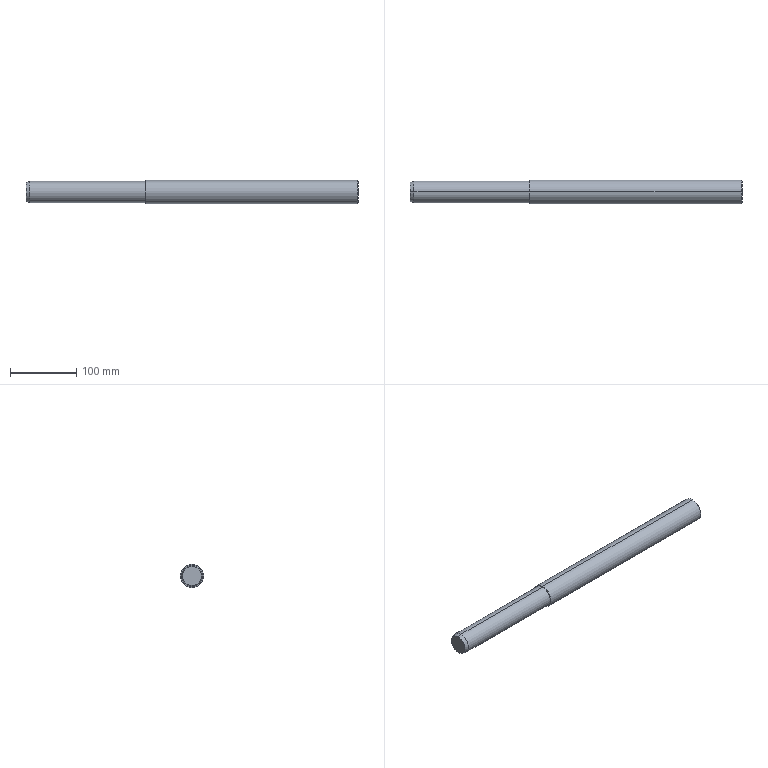Part | SolidWorks | features MBimport 1 | 1 solid | 20 faces | box 500 x 35 x 35 mm | volume 451710 mm3 | cone 8 | cylinder 8 | plane 4 | commonest cylinder face diameters 5 x2 6 x2 32 x2 35 x2
STEP:
#1=CARTESIAN_POINT('',(-0.025,10.786,1.92));
#2=VERTEX_POINT('',#1);
#3=CARTESIAN_POINT('',(0.,10.786,1.945));
#4=VERTEX_POINT('',#3);
#5=CARTESIAN_POINT('',(0.,10.786,1.945));
#6=DIRECTION('',(0.7071,0.,0.7071));
#7=VECTOR('',#6,1000.);
#8=LINE('',#5,#7);
#9=EDGE_CURVE('',#2,#4,#8,.T.);
#10=ORIENTED_EDGE('',*,*,#9,.F.);
#11=CARTESIAN_POINT('',(-0.025,10.786,-4.08));
#12=VERTEX_POINT('',#11);
#13=CARTESIAN_POINT('',(-0.025,10.786,-1.08));
#14=DIRECTION('',(1.,0.,0.));
#15=DIRECTION('',(0.,0.,-1.));
#16=AXIS2_PLACEMENT_3D('',#13,#14,#15);
#17=CIRCLE('',#16,3.);
#18=EDGE_CURVE('',#12,#2,#17,.T.);
#19=ORIENTED_EDGE('',*,*,#18,.F.);
#20=CARTESIAN_POINT('',(0.,10.786,-4.105));
#21=VERTEX_POINT('',#20);
#22=CARTESIAN_POINT('',(0.,10.786,-4.105));
#23=DIRECTION('',(0.7071,0.,-0.7071));
#24=VECTOR('',#23,1000.);
#25=LINE('',#22,#24);
#26=EDGE_CURVE('',#12,#21,#25,.T.);
#27=ORIENTED_EDGE('',*,*,#26,.T.);
#28=CARTESIAN_POINT('',(0.,10.786,-1.08));
#29=DIRECTION('',(1.,0.,0.));
#30=DIRECTION('',(0.,0.,-1.));
#31=AXIS2_PLACEMENT_3D('',#28,#29,#30);
#32=CIRCLE('',#31,3.025);
#33=EDGE_CURVE('',#21,#4,#32,.T.);
#34=ORIENTED_EDGE('',*,*,#33,.T.);
#35=EDGE_LOOP('',(#10,#19,#27,#34));
#36=FACE_OUTER_BOUND('',#35,.T.);
#37=CARTESIAN_POINT('',(0.,10.786,-1.08));
#38=DIRECTION('',(1.,0.,0.));
#39=DIRECTION('',(0.,0.,-1.));
#40=AXIS2_PLACEMENT_3D('',#37,#38,#39);
#41=CONICAL_SURFACE('',#40,3.025,0.7854);
#42=ADVANCED_FACE('',(#36),#41,.F.);
#43=CARTESIAN_POINT('',(-12.,10.786,1.92));
#44=VERTEX_POINT('',#43);
#45=CARTESIAN_POINT('',(0.,10.786,1.92));
#46=DIRECTION('',(1.,0.,0.));
#47=VECTOR('',#46,1000.);
#48=LINE('',#45,#47);
#49=EDGE_CURVE('',#44,#2,#48,.T.);
#50=ORIENTED_EDGE('',*,*,#49,.F.);
#51=CARTESIAN_POINT('',(-12.,10.786,-4.08));
#52=VERTEX_POINT('',#51);
#53=CARTESIAN_POINT('',(-12.,10.786,-1.08));
#54=DIRECTION('',(1.,0.,0.));
#55=DIRECTION('',(0.,0.,-1.));
#56=AXIS2_PLACEMENT_3D('',#53,#54,#55);
#57=CIRCLE('',#56,3.);
#58=EDGE_CURVE('',#52,#44,#57,.T.);
#59=ORIENTED_EDGE('',*,*,#58,.F.);
#60=CARTESIAN_POINT('',(0.,10.786,-4.08));
#61=DIRECTION('',(1.,0.,0.));
#62=VECTOR('',#61,1000.);
#63=LINE('',#60,#62);
#64=EDGE_CURVE('',#52,#12,#63,.T.);
#65=ORIENTED_EDGE('',*,*,#64,.T.);
#66=ORIENTED_EDGE('',*,*,#18,.T.);
#67=EDGE_LOOP('',(#50,#59,#65,#66));
#68=FACE_OUTER_BOUND('',#67,.T.);
#69=CARTESIAN_POINT('',(0.,10.786,-1.08));
#70=DIRECTION('',(1.,0.,0.));
#71=DIRECTION('',(0.,0.,-1.));
#72=AXIS2_PLACEMENT_3D('',#69,#70,#71);
#73=CYLINDRICAL_SURFACE('',#72,3.);
#74=ADVANCED_FACE('',(#68),#73,.F.);
#75=CARTESIAN_POINT('',(-12.,10.786,-3.58));
#76=VERTEX_POINT('',#75);
#77=CARTESIAN_POINT('',(-12.,10.786,1.42));
#78=VERTEX_POINT('',#77);
#79=CARTESIAN_POINT('',(-12.,10.786,-1.08));
#80=DIRECTION('',(1.,0.,0.));
#81=DIRECTION('',(0.,0.,-1.));
#82=AXIS2_PLACEMENT_3D('',#79,#80,#81);
#83=CIRCLE('',#82,2.5);
#84=EDGE_CURVE('',#76,#78,#83,.T.);
#85=ORIENTED_EDGE('',*,*,#84,.F.);
#86=CARTESIAN_POINT('',(-12.,10.786,-1.08));
#87=DIRECTION('',(1.,0.,0.));
#88=DIRECTION('',(0.,0.,-1.));
#89=AXIS2_PLACEMENT_3D('',#86,#87,#88);
#90=CIRCLE('',#89,2.5);
#91=EDGE_CURVE('',#78,#76,#90,.T.);
#92=ORIENTED_EDGE('',*,*,#91,.F.);
#93=EDGE_LOOP('',(#85,#92));
#94=FACE_BOUND('',#93,.T.);
#95=ORIENTED_EDGE('',*,*,#58,.T.);
#96=CARTESIAN_POINT('',(-12.,10.786,-1.08));
#97=DIRECTION('',(1.,0.,0.));
#98=DIRECTION('',(0.,0.,-1.));
#99=AXIS2_PLACEMENT_3D('',#96,#97,#98);
#100=CIRCLE('',#99,3.);
#101=EDGE_CURVE('',#44,#52,#100,.T.);
#102=ORIENTED_EDGE('',*,*,#101,.T.);
#103=EDGE_LOOP('',(#95,#102));
#104=FACE_OUTER_BOUND('',#103,.T.);
#105=CARTESIAN_POINT('',(-12.,13.286,-1.08));
#106=DIRECTION('',(-1.,0.,0.));
#107=DIRECTION('',(0.,0.,1.));
#108=AXIS2_PLACEMENT_3D('',#105,#106,#107);
#109=PLANE('',#108);
#110=ADVANCED_FACE('',(#94,#104),#109,.F.);
#111=CARTESIAN_POINT('',(-15.,10.786,1.42));
#112=VERTEX_POINT('',#111);
#113=CARTESIAN_POINT('',(0.,10.786,1.42));
#114=DIRECTION('',(1.,0.,0.));
#115=VECTOR('',#114,1000.);
#116=LINE('',#113,#115);
#117=EDGE_CURVE('',#112,#78,#116,.T.);
#118=ORIENTED_EDGE('',*,*,#117,.F.);
#119=CARTESIAN_POINT('',(-15.,10.786,-3.58));
#120=VERTEX_POINT('',#119);
#121=CARTESIAN_POINT('',(-15.,10.786,-1.08));
#122=DIRECTION('',(1.,0.,0.));
#123=DIRECTION('',(0.,0.,-1.));
#124=AXIS2_PLACEMENT_3D('',#121,#122,#123);
#125=CIRCLE('',#124,2.5);
#126=EDGE_CURVE('',#120,#112,#125,.T.);
#127=ORIENTED_EDGE('',*,*,#126,.F.);
#128=CARTESIAN_POINT('',(0.,10.786,-3.58));
#129=DIRECTION('',(1.,0.,0.));
#130=VECTOR('',#129,1000.);
#131=LINE('',#128,#130);
#132=EDGE_CURVE('',#120,#76,#131,.T.);
#133=ORIENTED_EDGE('',*,*,#132,.T.);
#134=ORIENTED_EDGE('',*,*,#84,.T.);
#135=EDGE_LOOP('',(#118,#127,#133,#134));
#136=FACE_OUTER_BOUND('',#135,.T.);
#137=CARTESIAN_POINT('',(0.,10.786,-1.08));
#138=DIRECTION('',(1.,0.,0.));
#139=DIRECTION('',(0.,0.,-1.));
#140=AXIS2_PLACEMENT_3D('',#137,#138,#139);
#141=CYLINDRICAL_SURFACE('',#140,2.5);
#142=ADVANCED_FACE('',(#136),#141,.F.);
#143=CARTESIAN_POINT('',(-16.502,10.786,-1.08));
#144=VERTEX_POINT('',#143);
#145=CARTESIAN_POINT('',(-15.,10.786,1.42));
#146=DIRECTION('',(0.515,0.,0.8572));
#147=VECTOR('',#146,1000.);
#148=LINE('',#145,#147);
#149=EDGE_CURVE('',#144,#112,#148,.T.);
#150=ORIENTED_EDGE('',*,*,#149,.F.);
#151=CARTESIAN_POINT('',(-15.,10.786,-3.58));
#152=DIRECTION('',(0.515,0.,-0.8572));
#153=VECTOR('',#152,1000.);
#154=LINE('',#151,#153);
#155=EDGE_CURVE('',#144,#120,#154,.T.);
#156=ORIENTED_EDGE('',*,*,#155,.T.);
#157=ORIENTED_EDGE('',*,*,#126,.T.);
#158=EDGE_LOOP('',(#150,#156,#157));
#159=FACE_OUTER_BOUND('',#158,.T.);
#160=CARTESIAN_POINT('',(-15.,10.786,-1.08));
#161=DIRECTION('',(1.,0.,0.));
#162=DIRECTION('',(0.,0.,-1.));
#163=AXIS2_PLACEMENT_3D('',#160,#161,#162);
#164=CONICAL_SURFACE('',#163,2.5,1.03);
#165=ADVANCED_FACE('',(#159),#164,.F.);
#166=CARTESIAN_POINT('',(0.,10.786,-17.58));
#167=VERTEX_POINT('',#166);
#168=CARTESIAN_POINT('',(-1.,10.786,-18.58));
#169=VERTEX_POINT('',#168);
#170=CARTESIAN_POINT('',(0.,10.786,-17.58));
#171=DIRECTION('',(-0.7071,0.,-0.7071));
#172=VECTOR('',#171,1000.);
#173=LINE('',#170,#172);
#174=EDGE_CURVE('',#167,#169,#173,.T.);
#175=ORIENTED_EDGE('',*,*,#174,.F.);
#176=CARTESIAN_POINT('',(0.,10.786,15.42));
#177=VERTEX_POINT('',#176);
#178=CARTESIAN_POINT('',(0.,10.786,-1.08));
#179=DIRECTION('',(1.,0.,0.));
#180=DIRECTION('',(0.,0.,-1.));
#181=AXIS2_PLACEMENT_3D('',#178,#179,#180);
#182=CIRCLE('',#181,16.5);
#183=EDGE_CURVE('',#177,#167,#182,.T.);
#184=ORIENTED_EDGE('',*,*,#183,.F.);
#185=CARTESIAN_POINT('',(-1.,10.786,16.42));
#186=VERTEX_POINT('',#185);
#187=CARTESIAN_POINT('',(0.,10.786,15.42));
#188=DIRECTION('',(-0.7071,0.,0.7071));
#189=VECTOR('',#188,1000.);
#190=LINE('',#187,#189);
#191=EDGE_CURVE('',#177,#186,#190,.T.);
#192=ORIENTED_EDGE('',*,*,#191,.T.);
#193=CARTESIAN_POINT('',(-1.,10.786,-1.08));
#194=DIRECTION('',(-1.,0.,0.));
#195=DIRECTION('',(0.,0.,-1.));
#196=AXIS2_PLACEMENT_3D('',#193,#194,#195);
#197=CIRCLE('',#196,17.5);
#198=EDGE_CURVE('',#169,#186,#197,.T.);
#199=ORIENTED_EDGE('',*,*,#198,.F.);
#200=EDGE_LOOP('',(#175,#184,#192,#199));
#201=FACE_OUTER_BOUND('',#200,.T.);
#202=CARTESIAN_POINT('',(0.,10.786,-1.08));
#203=DIRECTION('',(-1.,0.,0.));
#204=DIRECTION('',(0.,0.,1.));
#205=AXIS2_PLACEMENT_3D('',#202,#203,#204);
#206=CONICAL_SURFACE('',#205,16.5,0.7854);
#207=ADVANCED_FACE('',(#201),#206,.T.);
#208=CARTESIAN_POINT('',(-500.,10.786,13.313));
#209=VERTEX_POINT('',#208);
#210=CARTESIAN_POINT('',(-494.,10.786,14.92));
#211=VERTEX_POINT('',#210);
#212=CARTESIAN_POINT('',(-500.,10.786,13.313));
#213=DIRECTION('',(0.9659,0.,0.2588));
#214=VECTOR('',#213,1000.);
#215=LINE('',#212,#214);
#216=EDGE_CURVE('',#209,#211,#215,.T.);
#217=ORIENTED_EDGE('',*,*,#216,.F.);
#218=CARTESIAN_POINT('',(-500.,10.786,-15.472));
#219=VERTEX_POINT('',#218);
#220=CARTESIAN_POINT('',(-500.,10.786,-1.08));
#221=DIRECTION('',(-1.,0.,0.));
#222=DIRECTION('',(0.,0.,1.));
#223=AXIS2_PLACEMENT_3D('',#220,#221,#222);
#224=CIRCLE('',#223,14.392);
#225=EDGE_CURVE('',#219,#209,#224,.T.);
#226=ORIENTED_EDGE('',*,*,#225,.F.);
#227=CARTESIAN_POINT('',(-494.,10.786,-17.08));
#228=VERTEX_POINT('',#227);
#229=CARTESIAN_POINT('',(-500.,10.786,-15.472));
#230=DIRECTION('',(0.9659,0.,-0.2588));
#231=VECTOR('',#230,1000.);
#232=LINE('',#229,#231);
#233=EDGE_CURVE('',#219,#228,#232,.T.);
#234=ORIENTED_EDGE('',*,*,#233,.T.);
#235=CARTESIAN_POINT('',(-494.,10.786,-1.08));
#236=DIRECTION('',(1.,0.,0.));
#237=DIRECTION('',(0.,0.,1.));
#238=AXIS2_PLACEMENT_3D('',#235,#236,#237);
#239=CIRCLE('',#238,16.);
#240=EDGE_CURVE('',#211,#228,#239,.T.);
#241=ORIENTED_EDGE('',*,*,#240,.F.);
#242=EDGE_LOOP('',(#217,#226,#234,#241));
#243=FACE_OUTER_BOUND('',#242,.T.);
#244=CARTESIAN_POINT('',(-500.,10.786,-1.08));
#245=DIRECTION('',(1.,0.,0.));
#246=DIRECTION('',(0.,0.,-1.));
#247=AXIS2_PLACEMENT_3D('',#244,#245,#246);
#248=CONICAL_SURFACE('',#247,14.392,0.2618);
#249=ADVANCED_FACE('',(#243),#248,.T.);
#250=ORIENTED_EDGE('',*,*,#225,.T.);
#251=CARTESIAN_POINT('',(-500.,10.786,-1.08));
#252=DIRECTION('',(-1.,0.,0.));
#253=DIRECTION('',(0.,0.,1.));
#254=AXIS2_PLACEMENT_3D('',#251,#252,#253);
#255=CIRCLE('',#254,14.392);
#256=EDGE_CURVE('',#209,#219,#255,.T.);
#257=ORIENTED_EDGE('',*,*,#256,.T.);
#258=EDGE_LOOP('',(#250,#257));
#259=FACE_OUTER_BOUND('',#258,.T.);
#260=CARTESIAN_POINT('',(-500.,10.786,-1.08));
#261=DIRECTION('',(-1.,0.,0.));
#262=DIRECTION('',(0.,0.,1.));
#263=AXIS2_PLACEMENT_3D('',#260,#261,#262);
#264=PLANE('',#263);
#265=ADVANCED_FACE('',(#259),#264,.T.);
#266=CARTESIAN_POINT('',(-320.,10.786,14.92));
#267=VERTEX_POINT('',#266);
#268=CARTESIAN_POINT('',(-500.,10.786,14.92));
#269=DIRECTION('',(1.,0.,0.));
#270=VECTOR('',#269,1000.);
#271=LINE('',#268,#270);
#272=EDGE_CURVE('',#211,#267,#271,.T.);
#273=ORIENTED_EDGE('',*,*,#272,.F.);
#274=ORIENTED_EDGE('',*,*,#240,.T.);
#275=CARTESIAN_POINT('',(-320.,10.786,-17.08));
#276=VERTEX_POINT('',#275);
#277=CARTESIAN_POINT('',(-500.,10.786,-17.08));
#278=DIRECTION('',(1.,0.,0.));
#279=VECTOR('',#278,1000.);
#280=LINE('',#277,#279);
#281=EDGE_CURVE('',#228,#276,#280,.T.);
#282=ORIENTED_EDGE('',*,*,#281,.T.);
#283=CARTESIAN_POINT('',(-320.,10.786,-1.08));
#284=DIRECTION('',(-1.,0.,0.));
#285=DIRECTION('',(0.,0.,1.));
#286=AXIS2_PLACEMENT_3D('',#283,#284,#285);
#287=CIRCLE('',#286,16.);
#288=EDGE_CURVE('',#276,#267,#287,.T.);
#289=ORIENTED_EDGE('',*,*,#288,.T.);
#290=EDGE_LOOP('',(#273,#274,#282,#289));
#291=FACE_OUTER_BOUND('',#290,.T.);
#292=CARTESIAN_POINT('',(-500.,10.786,-1.08));
#293=DIRECTION('',(1.,0.,0.));
#294=DIRECTION('',(0.,0.,-1.));
#295=AXIS2_PLACEMENT_3D('',#292,#293,#294);
#296=CYLINDRICAL_SURFACE('',#295,16.);
#297=ADVANCED_FACE('',(#291),#296,.T.);
#298=ORIENTED_EDGE('',*,*,#33,.F.);
#299=CARTESIAN_POINT('',(0.,10.786,-1.08));
#300=DIRECTION('',(1.,0.,0.));
#301=DIRECTION('',(0.,0.,-1.));
#302=AXIS2_PLACEMENT_3D('',#299,#300,#301);
#303=CIRCLE('',#302,3.025);
#304=EDGE_CURVE('',#4,#21,#303,.T.);
#305=ORIENTED_EDGE('',*,*,#304,.F.);
#306=EDGE_LOOP('',(#298,#305));
#307=FACE_BOUND('',#306,.T.);
#308=ORIENTED_EDGE('',*,*,#183,.T.);
#309=CARTESIAN_POINT('',(0.,10.786,-1.08));
#310=DIRECTION('',(1.,0.,0.));
#311=DIRECTION('',(0.,0.,-1.));
#312=AXIS2_PLACEMENT_3D('',#309,#310,#311);
#313=CIRCLE('',#312,16.5);
#314=EDGE_CURVE('',#167,#177,#313,.T.);
#315=ORIENTED_EDGE('',*,*,#314,.T.);
#316=EDGE_LOOP('',(#308,#315));
#317=FACE_OUTER_BOUND('',#316,.T.);
#318=CARTESIAN_POINT('',(0.,10.786,-1.08));
#319=DIRECTION('',(1.,0.,0.));
#320=DIRECTION('',(0.,1.,0.));
#321=AXIS2_PLACEMENT_3D('',#318,#319,#320);
#322=PLANE('',#321);
#323=ADVANCED_FACE('',(#307,#317),#322,.T.);
#324=ORIENTED_EDGE('',*,*,#288,.F.);
#325=CARTESIAN_POINT('',(-320.,10.786,-1.08));
#326=DIRECTION('',(-1.,0.,0.));
#327=DIRECTION('',(0.,0.,1.));
#328=AXIS2_PLACEMENT_3D('',#325,#326,#327);
#329=CIRCLE('',#328,16.);
#330=EDGE_CURVE('',#267,#276,#329,.T.);
#331=ORIENTED_EDGE('',*,*,#330,.F.);
#332=EDGE_LOOP('',(#324,#331));
#333=FACE_BOUND('',#332,.T.);
#334=CARTESIAN_POINT('',(-320.,10.786,-18.58));
#335=VERTEX_POINT('',#334);
#336=CARTESIAN_POINT('',(-320.,10.786,16.42));
#337=VERTEX_POINT('',#336);
#338=CARTESIAN_POINT('',(-320.,10.786,-1.08));
#339=DIRECTION('',(1.,0.,0.));
#340=DIRECTION('',(0.,0.,-1.));
#341=AXIS2_PLACEMENT_3D('',#338,#339,#340);
#342=CIRCLE('',#341,17.5);
#343=EDGE_CURVE('',#335,#337,#342,.T.);
#344=ORIENTED_EDGE('',*,*,#343,.F.);
#345=CARTESIAN_POINT('',(-320.,10.786,-1.08));
#346=DIRECTION('',(1.,0.,0.));
#347=DIRECTION('',(0.,0.,-1.));
#348=AXIS2_PLACEMENT_3D('',#345,#346,#347);
#349=CIRCLE('',#348,17.5);
#350=EDGE_CURVE('',#337,#335,#349,.T.);
#351=ORIENTED_EDGE('',*,*,#350,.F.);
#352=EDGE_LOOP('',(#344,#351));
#353=FACE_OUTER_BOUND('',#352,.T.);
#354=CARTESIAN_POINT('',(-320.,10.786,-1.08));
#355=DIRECTION('',(1.,0.,0.));
#356=DIRECTION('',(0.,1.,0.));
#357=AXIS2_PLACEMENT_3D('',#354,#355,#356);
#358=PLANE('',#357);
#359=ADVANCED_FACE('',(#333,#353),#358,.F.);
#360=CARTESIAN_POINT('',(-320.,10.786,16.42));
#361=DIRECTION('',(1.,0.,0.));
#362=VECTOR('',#361,1000.);
#363=LINE('',#360,#362);
#364=EDGE_CURVE('',#337,#186,#363,.T.);
#365=ORIENTED_EDGE('',*,*,#364,.F.);
#366=ORIENTED_EDGE('',*,*,#350,.T.);
#367=CARTESIAN_POINT('',(-320.,10.786,-18.58));
#368=DIRECTION('',(1.,0.,0.));
#369=VECTOR('',#368,1000.);
#370=LINE('',#367,#369);
#371=EDGE_CURVE('',#335,#169,#370,.T.);
#372=ORIENTED_EDGE('',*,*,#371,.T.);
#373=ORIENTED_EDGE('',*,*,#198,.T.);
#374=EDGE_LOOP('',(#365,#366,#372,#373));
#375=FACE_OUTER_BOUND('',#374,.T.);
#376=CARTESIAN_POINT('',(-320.,10.786,-1.08));
#377=DIRECTION('',(1.,0.,0.));
#378=DIRECTION('',(0.,0.,-1.));
#379=AXIS2_PLACEMENT_3D('',#376,#377,#378);
#380=CYLINDRICAL_SURFACE('',#379,17.5);
#381=ADVANCED_FACE('',(#375),#380,.T.);
#382=ORIENTED_EDGE('',*,*,#343,.T.);
#383=ORIENTED_EDGE('',*,*,#364,.T.);
#384=CARTESIAN_POINT('',(-1.,10.786,-1.08));
#385=DIRECTION('',(-1.,0.,0.));
#386=DIRECTION('',(0.,0.,-1.));
#387=AXIS2_PLACEMENT_3D('',#384,#385,#386);
#388=CIRCLE('',#387,17.5);
#389=EDGE_CURVE('',#186,#169,#388,.T.);
#390=ORIENTED_EDGE('',*,*,#389,.T.);
#391=ORIENTED_EDGE('',*,*,#371,.F.);
#392=EDGE_LOOP('',(#382,#383,#390,#391));
#393=FACE_OUTER_BOUND('',#392,.T.);
#394=CARTESIAN_POINT('',(-320.,10.786,-1.08));
#395=DIRECTION('',(1.,0.,0.));
#396=DIRECTION('',(0.,0.,-1.));
#397=AXIS2_PLACEMENT_3D('',#394,#395,#396);
#398=CYLINDRICAL_SURFACE('',#397,17.5);
#399=ADVANCED_FACE('',(#393),#398,.T.);
#400=CARTESIAN_POINT('',(-494.,10.786,-1.08));
#401=DIRECTION('',(1.,0.,0.));
#402=DIRECTION('',(0.,0.,1.));
#403=AXIS2_PLACEMENT_3D('',#400,#401,#402);
#404=CIRCLE('',#403,16.);
#405=EDGE_CURVE('',#228,#211,#404,.T.);
#406=ORIENTED_EDGE('',*,*,#405,.T.);
#407=ORIENTED_EDGE('',*,*,#272,.T.);
#408=ORIENTED_EDGE('',*,*,#330,.T.);
#409=ORIENTED_EDGE('',*,*,#281,.F.);
#410=EDGE_LOOP('',(#406,#407,#408,#409));
#411=FACE_OUTER_BOUND('',#410,.T.);
#412=CARTESIAN_POINT('',(-500.,10.786,-1.08));
#413=DIRECTION('',(1.,0.,0.));
#414=DIRECTION('',(0.,0.,-1.));
#415=AXIS2_PLACEMENT_3D('',#412,#413,#414);
#416=CYLINDRICAL_SURFACE('',#415,16.);
#417=ADVANCED_FACE('',(#411),#416,.T.);
#418=ORIENTED_EDGE('',*,*,#256,.F.);
#419=ORIENTED_EDGE('',*,*,#216,.T.);
#420=ORIENTED_EDGE('',*,*,#405,.F.);
#421=ORIENTED_EDGE('',*,*,#233,.F.);
#422=EDGE_LOOP('',(#418,#419,#420,#421));
#423=FACE_OUTER_BOUND('',#422,.T.);
#424=CARTESIAN_POINT('',(-500.,10.786,-1.08));
#425=DIRECTION('',(1.,0.,0.));
#426=DIRECTION('',(0.,0.,-1.));
#427=AXIS2_PLACEMENT_3D('',#424,#425,#426);
#428=CONICAL_SURFACE('',#427,14.392,0.2618);
#429=ADVANCED_FACE('',(#423),#428,.T.);
#430=ORIENTED_EDGE('',*,*,#314,.F.);
#431=ORIENTED_EDGE('',*,*,#174,.T.);
#432=ORIENTED_EDGE('',*,*,#389,.F.);
#433=ORIENTED_EDGE('',*,*,#191,.F.);
#434=EDGE_LOOP('',(#430,#431,#432,#433));
#435=FACE_OUTER_BOUND('',#434,.T.);
#436=CARTESIAN_POINT('',(0.,10.786,-1.08));
#437=DIRECTION('',(-1.,0.,0.));
#438=DIRECTION('',(0.,0.,1.));
#439=AXIS2_PLACEMENT_3D('',#436,#437,#438);
#440=CONICAL_SURFACE('',#439,16.5,0.7854);
#441=ADVANCED_FACE('',(#435),#440,.T.);
#442=ORIENTED_EDGE('',*,*,#155,.F.);
#443=ORIENTED_EDGE('',*,*,#149,.T.);
#444=CARTESIAN_POINT('',(-15.,10.786,-1.08));
#445=DIRECTION('',(1.,0.,0.));
#446=DIRECTION('',(0.,0.,-1.));
#447=AXIS2_PLACEMENT_3D('',#444,#445,#446);
#448=CIRCLE('',#447,2.5);
#449=EDGE_CURVE('',#112,#120,#448,.T.);
#450=ORIENTED_EDGE('',*,*,#449,.T.);
#451=EDGE_LOOP('',(#442,#443,#450));
#452=FACE_OUTER_BOUND('',#451,.T.);
#453=CARTESIAN_POINT('',(-15.,10.786,-1.08));
#454=DIRECTION('',(1.,0.,0.));
#455=DIRECTION('',(0.,0.,-1.));
#456=AXIS2_PLACEMENT_3D('',#453,#454,#455);
#457=CONICAL_SURFACE('',#456,2.5,1.03);
#458=ADVANCED_FACE('',(#452),#457,.F.);
#459=ORIENTED_EDGE('',*,*,#449,.F.);
#460=ORIENTED_EDGE('',*,*,#117,.T.);
#461=ORIENTED_EDGE('',*,*,#91,.T.);
#462=ORIENTED_EDGE('',*,*,#132,.F.);
#463=EDGE_LOOP('',(#459,#460,#461,#462));
#464=FACE_OUTER_BOUND('',#463,.T.);
#465=CARTESIAN_POINT('',(0.,10.786,-1.08));
#466=DIRECTION('',(1.,0.,0.));
#467=DIRECTION('',(0.,0.,-1.));
#468=AXIS2_PLACEMENT_3D('',#465,#466,#467);
#469=CYLINDRICAL_SURFACE('',#468,2.5);
#470=ADVANCED_FACE('',(#464),#469,.F.);
#471=ORIENTED_EDGE('',*,*,#101,.F.);
#472=ORIENTED_EDGE('',*,*,#49,.T.);
#473=CARTESIAN_POINT('',(-0.025,10.786,-1.08));
#474=DIRECTION('',(1.,0.,0.));
#475=DIRECTION('',(0.,0.,-1.));
#476=AXIS2_PLACEMENT_3D('',#473,#474,#475);
#477=CIRCLE('',#476,3.);
#478=EDGE_CURVE('',#2,#12,#477,.T.);
#479=ORIENTED_EDGE('',*,*,#478,.T.);
#480=ORIENTED_EDGE('',*,*,#64,.F.);
#481=EDGE_LOOP('',(#471,#472,#479,#480));
#482=FACE_OUTER_BOUND('',#481,.T.);
#483=CARTESIAN_POINT('',(0.,10.786,-1.08));
#484=DIRECTION('',(1.,0.,0.));
#485=DIRECTION('',(0.,0.,-1.));
#486=AXIS2_PLACEMENT_3D('',#483,#484,#485);
#487=CYLINDRICAL_SURFACE('',#486,3.);
#488=ADVANCED_FACE('',(#482),#487,.F.);
#489=ORIENTED_EDGE('',*,*,#478,.F.);
#490=ORIENTED_EDGE('',*,*,#9,.T.);
#491=ORIENTED_EDGE('',*,*,#304,.T.);
#492=ORIENTED_EDGE('',*,*,#26,.F.);
#493=EDGE_LOOP('',(#489,#490,#491,#492));
#494=FACE_OUTER_BOUND('',#493,.T.);
#495=CARTESIAN_POINT('',(0.,10.786,-1.08));
#496=DIRECTION('',(1.,0.,0.));
#497=DIRECTION('',(0.,0.,-1.));
#498=AXIS2_PLACEMENT_3D('',#495,#496,#497);
#499=CONICAL_SURFACE('',#498,3.025,0.7854);
#500=ADVANCED_FACE('',(#494),#499,.F.);
#501=CLOSED_SHELL('',(#42,#74,#110,#142,#165,#207,#249,#265,#297,#323,#359,#381,#399,#417,#429,#441,#458,#470,#488,#500));
#502=MANIFOLD_SOLID_BREP('',#501);
#503=CARTESIAN_POINT('',(0.,0.,0.));
#504=DIRECTION('',(0.,0.,1.));
#505=DIRECTION('',(1.,0.,0.));
#506=AXIS2_PLACEMENT_3D('',#503,#504,#505);
#507=(LENGTH_UNIT()NAMED_UNIT(*)SI_UNIT(.MILLI.,.METRE.));
#508=UNCERTAINTY_MEASURE_WITH_UNIT(LENGTH_MEASURE(0.00001),#507,'','');
#509=(NAMED_UNIT(*)PLANE_ANGLE_UNIT()SI_UNIT($,.RADIAN.));
#510=(NAMED_UNIT(*)SI_UNIT($,.STERADIAN.)SOLID_ANGLE_UNIT());
#511=(GEOMETRIC_REPRESENTATION_CONTEXT(3)GLOBAL_UNCERTAINTY_ASSIGNED_CONTEXT((#508))GLOBAL_UNIT_ASSIGNED_CONTEXT((#507,#509,#510))REPRESENTATION_CONTEXT('',''));
#512=ADVANCED_BREP_SHAPE_REPRESENTATION('',(#502,#506),#511);